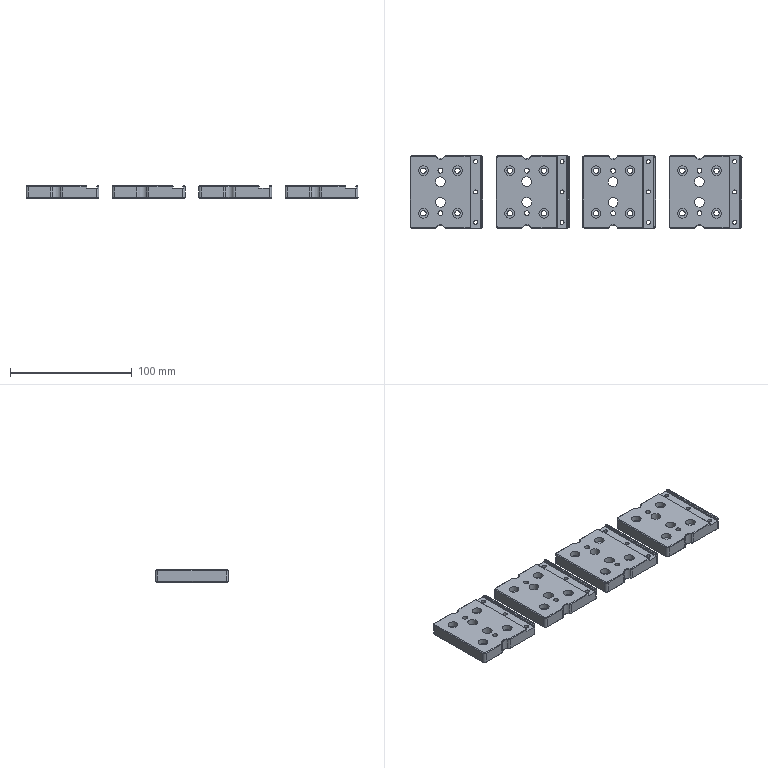Part | 4 solids | 332 faces | box 273 x 60 x 10 mm | volume 127813 mm3 | plane 152 | cylinder 100 | cone 80 | commonest cylinder face diameters 4 x40 8 x32 4.5 x16 3.3 x12